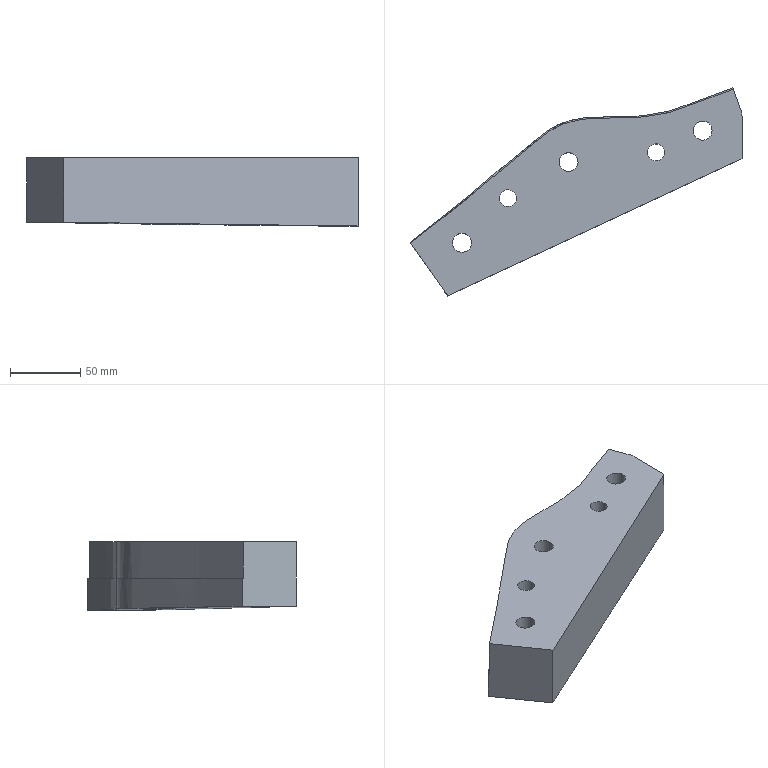Part | NX | features solid 2 | 1 solid | 27 faces | box 236.188 x 148.081 x 48.904 mm | volume 669282 mm3 | plane 12 | cylinder 11 | spline 4 | commonest cylinder face diameters 13.5 x3 19.5 x3 12 x2 13 x2 30 x1